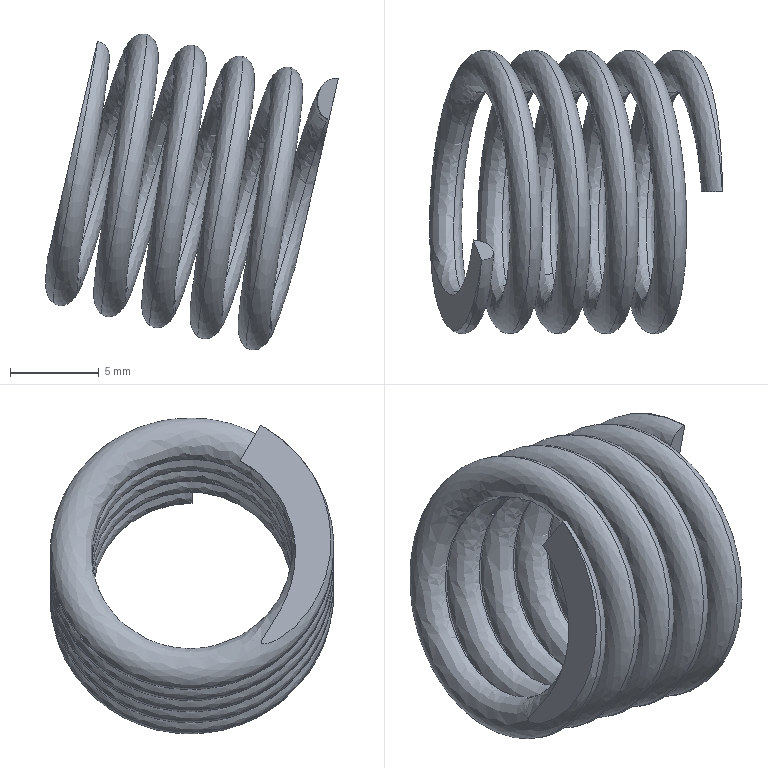Part | SolidWorks | features BaseBody 1 | 1 solid | 6 faces | box 16.505 x 16.005 x 17.799 mm | volume 676.72 mm3 | plane 4 | spline 2